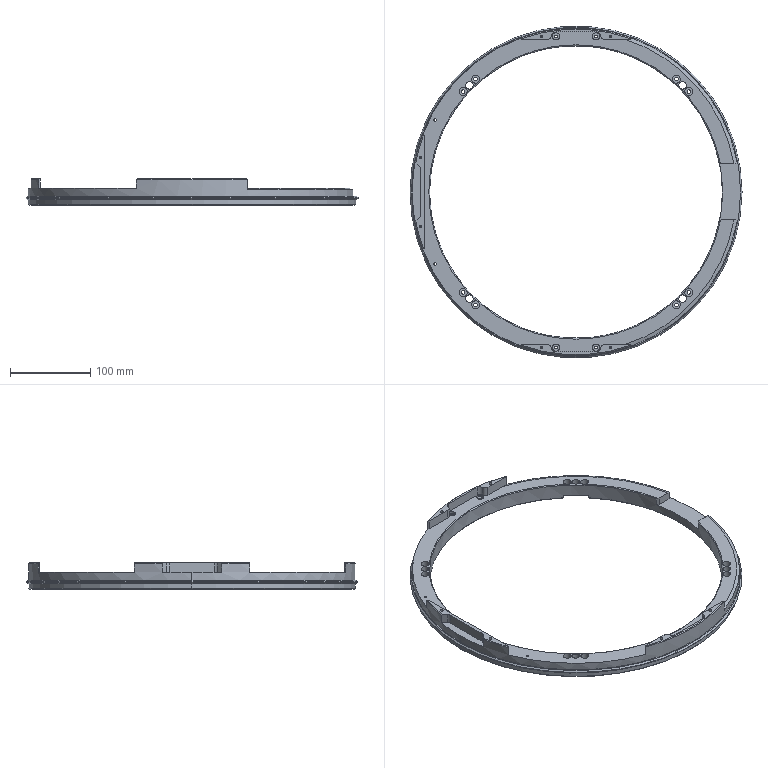Part | NX | features BREP 1 | 1 solid | 264 faces | box 415 x 415 x 33 mm | volume 391645 mm3 | cylinder 162 | plane 70 | cone 32 | commonest cylinder face diameters 12 x36 3.3 x24 10 x22 4.5 x16 374 x13 398 x13